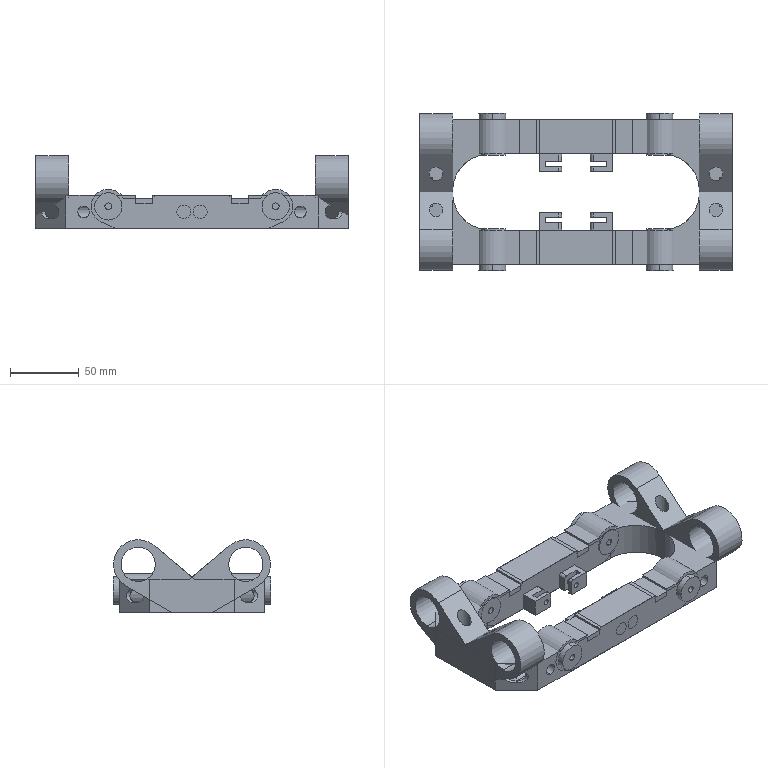NC program | Mastercam | posted with a generic post | part box 228 x 114.503 x 53 mm
Lines 2708 to 3806 of 27132:
(10 FEM |TOOL - 10|DIA. OFF. - 10|LEN. - 10|TOOL DIA. - 10.)
N5468 T10 M6
N5470 G0 G54 G90 X14.273 Y-4.51 C0. B0. S8000 M3
N5472 G43 H10 Z50.
N5474 Z5.
N5476 G1 Z-.5 F600.
N5478 Y-3.51 F4000.
N5480 G3 X13.273 Y-2.51 I-1.
N5482 G1 X3.684
N5484 X-3.024 Y-8.139
N5486 G3 X-3.381 Y-8.905 I.642 J-.766
N5488 X-3.148 Y-9.548 I.999
N5490 G1 X-2.505 Y-10.314
N5492 X14.273 Y-4.51
N5494 Z-1. F600.
N5496 Y-3.51 F4000.
N5498 G3 X13.273 Y-2.51 I-1.
N5500 G1 X3.684
N5502 X-3.024 Y-8.139
N5504 G3 X-3.381 Y-8.905 I.642 J-.766
N5506 X-3.148 Y-9.548 I.999
N5508 G1 X-2.505 Y-10.314
N5510 X14.273 Y-4.51
N5512 Z-1.5 F600.
N5514 Y-3.51 F4000.
N5516 G3 X13.273 Y-2.51 I-1.
N5518 G1 X3.684
N5520 X-3.024 Y-8.139
N5522 G3 X-3.381 Y-8.905 I.642 J-.766
N5524 X-3.148 Y-9.548 I.999
N5526 G1 X-2.505 Y-10.314
N5528 X14.273 Y-4.51
N5530 Z-2. F600.
N5532 Y-3.51 F4000.
N5534 G3 X13.273 Y-2.51 I-1.
N5536 G1 X3.684
N5538 X-3.024 Y-8.139
N5540 G3 X-3.381 Y-8.905 I.642 J-.766
N5542 X-3.148 Y-9.548 I.999
N5544 G1 X-2.505 Y-10.314
N5546 X14.273 Y-4.51
N5548 Z-2.5 F600.
N5550 Y-3.51 F4000.
N5552 G3 X13.273 Y-2.51 I-1.
N5554 G1 X3.684
N5556 X-3.024 Y-8.139
N5558 G3 X-3.381 Y-8.905 I.642 J-.766
N5560 X-3.148 Y-9.548 I.999
N5562 G1 X-2.505 Y-10.314
N5564 X14.273 Y-4.51
N5566 Z-3. F600.
N5568 Y-3.51 F4000.
N5570 G3 X13.273 Y-2.51 I-1.
N5572 G1 X3.684
N5574 X-3.024 Y-8.139
N5576 G3 X-3.381 Y-8.905 I.642 J-.766
N5578 X-3.148 Y-9.548 I.999
N5580 G1 X-2.505 Y-10.314
N5582 X14.273 Y-4.51
N5584 Z-3.5 F600.
N5586 Y-3.51 F4000.
N5588 G3 X13.273 Y-2.51 I-1.
N5590 G1 X3.684
N5592 X-3.024 Y-8.139
N5594 G3 X-3.381 Y-8.905 I.642 J-.766
N5596 X-3.148 Y-9.548 I.999
N5598 G1 X-2.505 Y-10.314
N5600 X14.273 Y-4.51
N5602 Z-4. F600.
N5604 Y-3.51 F4000.
N5606 G3 X13.273 Y-2.51 I-1.
N5608 G1 X3.684
N5610 X-3.024 Y-8.139
N5612 G3 X-3.381 Y-8.905 I.642 J-.766
N5614 X-3.148 Y-9.548 I.999
N5616 G1 X-2.505 Y-10.314
N5618 X14.273 Y-4.51
N5620 Z-4.5 F600.
N5622 Y-3.51 F4000.
N5624 G3 X13.273 Y-2.51 I-1.
N5626 G1 X3.684
N5628 X-3.024 Y-8.139
N5630 G3 X-3.381 Y-8.905 I.642 J-.766
N5632 X-3.148 Y-9.548 I.999
N5634 G1 X-2.505 Y-10.314
N5636 X14.273 Y-4.51
N5638 Z-5. F600.
N5640 Y-3.51 F4000.
N5642 G3 X13.273 Y-2.51 I-1.
N5644 G1 X3.684
N5646 X-3.024 Y-8.139
N5648 G3 X-3.381 Y-8.905 I.642 J-.766
N5650 X-3.148 Y-9.548 I.999
N5652 G1 X-2.505 Y-10.314
N5654 X14.273 Y-4.51
N5656 Z-5.5 F600.
N5658 Y-3.51 F4000.
N5660 G3 X13.273 Y-2.51 I-1.
N5662 G1 X3.684
N5664 X-3.024 Y-8.139
N5666 G3 X-3.381 Y-8.905 I.642 J-.766
N5668 X-3.148 Y-9.548 I.999
N5670 G1 X-2.505 Y-10.314
N5672 X14.273 Y-4.51
N5674 Z-6. F600.
N5676 Y-3.51 F4000.
N5678 G3 X13.273 Y-2.51 I-1.
N5680 G1 X3.684
N5682 X-3.024 Y-8.139
N5684 G3 X-3.381 Y-8.905 I.642 J-.766
N5686 X-3.148 Y-9.548 I.999
N5688 G1 X-2.505 Y-10.314
N5690 X14.273 Y-4.51
N5692 Z-6.5 F600.
N5694 Y-3.51 F4000.
N5696 G3 X13.273 Y-2.51 I-1.
N5698 G1 X3.684
N5700 X-3.024 Y-8.139
N5702 G3 X-3.381 Y-8.905 I.642 J-.766
N5704 X-3.148 Y-9.548 I.999
N5706 G1 X-2.505 Y-10.314
N5708 X14.273 Y-4.51
N5710 Z-7. F600.
N5712 Y-3.51 F4000.
N5714 G3 X13.273 Y-2.51 I-1.
N5716 G1 X3.684
N5718 X-3.024 Y-8.139
N5720 G3 X-3.381 Y-8.905 I.642 J-.766
N5722 X-3.148 Y-9.548 I.999
N5724 G1 X-2.505 Y-10.314
N5726 X14.273 Y-4.51
N5728 Z-7.5 F600.
N5730 Y-3.51 F4000.
N5732 G3 X13.273 Y-2.51 I-1.
N5734 G1 X3.684
N5736 X-3.024 Y-8.139
N5738 G3 X-3.381 Y-8.905 I.642 J-.766
N5740 X-3.148 Y-9.548 I.999
N5742 G1 X-2.505 Y-10.314
N5744 X14.273 Y-4.51
N5746 Z-8. F600.
N5748 Y-3.51 F4000.
N5750 G3 X13.273 Y-2.51 I-1.
N5752 G1 X3.684
N5754 X-3.024 Y-8.139
N5756 G3 X-3.381 Y-8.905 I.642 J-.766
N5758 X-3.148 Y-9.548 I.999
N5760 G1 X-2.505 Y-10.314
N5762 X14.273 Y-4.51
N5764 Z-8.5 F600.
N5766 Y-3.51 F4000.
N5768 G3 X13.273 Y-2.51 I-1.
N5770 G1 X3.684
N5772 X-3.024 Y-8.139
N5774 G3 X-3.381 Y-8.905 I.642 J-.766
N5776 X-3.148 Y-9.548 I.999
N5778 G1 X-2.505 Y-10.314
N5780 X14.273 Y-4.51
N5782 Z-9. F600.
N5784 Y-3.51 F4000.
N5786 G3 X13.273 Y-2.51 I-1.
N5788 G1 X3.684
N5790 X-3.024 Y-8.139
N5792 G3 X-3.381 Y-8.905 I.642 J-.766
N5794 X-3.148 Y-9.548 I.999
N5796 G1 X-2.505 Y-10.314
N5798 X14.273 Y-4.51
N5800 Z-9.5 F600.
N5802 Y-3.51 F4000.
N5804 G3 X13.273 Y-2.51 I-1.
N5806 G1 X3.684
N5808 X-3.024 Y-8.139
N5810 G3 X-3.381 Y-8.905 I.642 J-.766
N5812 X-3.148 Y-9.548 I.999
N5814 G1 X-2.505 Y-10.314
N5816 X14.273 Y-4.51
N5818 Z-10. F600.
N5820 Y-3.51 F4000.
N5822 G3 X13.273 Y-2.51 I-1.
N5824 G1 X3.684
N5826 X-3.024 Y-8.139
N5828 G3 X-3.381 Y-8.905 I.642 J-.766
N5830 X-3.148 Y-9.548 I.999
N5832 G1 X-2.505 Y-10.314
N5834 X14.273 Y-4.51
N5836 Z-10.5 F600.
N5838 Y-3.51 F4000.
N5840 G3 X13.273 Y-2.51 I-1.
N5842 G1 X3.684
N5844 X-3.024 Y-8.139
N5846 G3 X-3.381 Y-8.905 I.642 J-.766
N5848 X-3.148 Y-9.548 I.999
N5850 G1 X-2.505 Y-10.314
N5852 X14.273 Y-4.51
N5854 Z-11. F600.
N5856 Y-3.51 F4000.
N5858 G3 X13.273 Y-2.51 I-1.
N5860 G1 X3.684
N5862 X-3.024 Y-8.139
N5864 G3 X-3.381 Y-8.905 I.642 J-.766
N5866 X-3.148 Y-9.548 I.999
N5868 G1 X-2.505 Y-10.314
N5870 X14.273 Y-4.51
N5872 Z-11.5 F600.
N5874 Y-3.51 F4000.
N5876 G3 X13.273 Y-2.51 I-1.
N5878 G1 X3.684
N5880 X-3.024 Y-8.139
N5882 G3 X-3.381 Y-8.905 I.642 J-.766
N5884 X-3.148 Y-9.548 I.999
N5886 G1 X-2.505 Y-10.314
N5888 X14.273 Y-4.51
N5890 Z-12. F600.
N5892 Y-3.51 F4000.
N5894 G3 X13.273 Y-2.51 I-1.
N5896 G1 X3.684
N5898 X-3.024 Y-8.139
N5900 G3 X-3.381 Y-8.905 I.642 J-.766
N5902 X-3.148 Y-9.548 I.999
N5904 G1 X-2.505 Y-10.314
N5906 X14.273 Y-4.51
N5908 Z-12.5 F600.
N5910 Y-3.51 F4000.
N5912 G3 X13.273 Y-2.51 I-1.
N5914 G1 X3.684
N5916 X-3.024 Y-8.139
N5918 G3 X-3.381 Y-8.905 I.642 J-.766
N5920 X-3.148 Y-9.548 I.999
N5922 G1 X-2.505 Y-10.314
N5924 X14.273 Y-4.51
N5926 Z-13. F600.
N5928 Y-3.51 F4000.
N5930 G3 X13.273 Y-2.51 I-1.
N5932 G1 X3.684
N5934 X-3.024 Y-8.139
N5936 G3 X-3.381 Y-8.905 I.642 J-.766
N5938 X-3.148 Y-9.548 I.999
N5940 G1 X-2.505 Y-10.314
N5942 X14.273 Y-4.51
N5944 Z-13.5 F600.
N5946 Y-3.51 F4000.
N5948 G3 X13.273 Y-2.51 I-1.
N5950 G1 X3.684
N5952 X-3.024 Y-8.139
N5954 G3 X-3.381 Y-8.905 I.642 J-.766
N5956 X-3.148 Y-9.548 I.999
N5958 G1 X-2.505 Y-10.314
N5960 X14.273 Y-4.51
N5962 Z-14. F600.
N5964 Y-3.51 F4000.
N5966 G3 X13.273 Y-2.51 I-1.
N5968 G1 X3.684
N5970 X-3.024 Y-8.139
N5972 G3 X-3.381 Y-8.905 I.642 J-.766
N5974 X-3.148 Y-9.548 I.999
N5976 G1 X-2.505 Y-10.314
N5978 X14.273 Y-4.51
N5980 Z-14.5 F600.
N5982 Y-3.51 F4000.
N5984 G3 X13.273 Y-2.51 I-1.
N5986 G1 X3.684
N5988 X-3.024 Y-8.139
N5990 G3 X-3.381 Y-8.905 I.642 J-.766
N5992 X-3.148 Y-9.548 I.999
N5994 G1 X-2.505 Y-10.314
N5996 X14.273 Y-4.51
N5998 Z-15. F600.
N6000 Y-3.51 F4000.
N6002 G3 X13.273 Y-2.51 I-1.
N6004 G1 X3.684
N6006 X-3.024 Y-8.139
N6008 G3 X-3.381 Y-8.905 I.642 J-.766
N6010 X-3.148 Y-9.548 I.999
N6012 G1 X-2.505 Y-10.314
N6014 X14.273 Y-4.51
N6016 Z-15.5 F600.
N6018 Y-3.51 F4000.
N6020 G3 X13.273 Y-2.51 I-1.
N6022 G1 X3.684
N6024 X-3.024 Y-8.139
N6026 G3 X-3.381 Y-8.905 I.642 J-.766
N6028 X-3.148 Y-9.548 I.999
N6030 G1 X-2.505 Y-10.314
N6032 X14.273 Y-4.51
N6034 Z-16. F600.
N6036 Y-3.51 F4000.
N6038 G3 X13.273 Y-2.51 I-1.
N6040 G1 X3.684
N6042 X-3.024 Y-8.139
N6044 G3 X-3.381 Y-8.905 I.642 J-.766
N6046 X-3.148 Y-9.548 I.999
N6048 G1 X-2.505 Y-10.314
N6050 X14.273 Y-4.51
N6052 Z-16.5 F600.
N6054 Y-3.51 F4000.
N6056 G3 X13.273 Y-2.51 I-1.
N6058 G1 X3.684
N6060 X-3.024 Y-8.139
N6062 G3 X-3.381 Y-8.905 I.642 J-.766
N6064 X-3.148 Y-9.548 I.999
N6066 G1 X-2.505 Y-10.314
N6068 X14.273 Y-4.51
N6070 Z-17. F600.
N6072 Y-3.51 F4000.
N6074 G3 X13.273 Y-2.51 I-1.
N6076 G1 X3.684
N6078 X-3.024 Y-8.139
N6080 G3 X-3.381 Y-8.905 I.642 J-.766
N6082 X-3.148 Y-9.548 I.999
N6084 G1 X-2.505 Y-10.314
N6086 X14.273 Y-4.51
N6088 Z-17.5 F600.
N6090 Y-3.51 F4000.
N6092 G3 X13.273 Y-2.51 I-1.
N6094 G1 X3.684
N6096 X-3.024 Y-8.139
N6098 G3 X-3.381 Y-8.905 I.642 J-.766
N6100 X-3.148 Y-9.548 I.999
N6102 G1 X-2.505 Y-10.314
N6104 X14.273 Y-4.51
N6106 Z-18. F600.
N6108 Y-3.51 F4000.
N6110 G3 X13.273 Y-2.51 I-1.
N6112 G1 X3.684
N6114 X-3.024 Y-8.139
N6116 G3 X-3.381 Y-8.905 I.642 J-.766
N6118 X-3.148 Y-9.548 I.999
N6120 G1 X-2.505 Y-10.314
N6122 X14.273 Y-4.51
N6124 Z-18.5 F600.
N6126 Y-3.51 F4000.
N6128 G3 X13.273 Y-2.51 I-1.
N6130 G1 X3.684
N6132 X-3.024 Y-8.139
N6134 G3 X-3.381 Y-8.905 I.642 J-.766
N6136 X-3.148 Y-9.548 I.999
N6138 G1 X-2.505 Y-10.314
N6140 X14.273 Y-4.51
N6142 Z-19. F600.
N6144 Y-3.51 F4000.
N6146 G3 X13.273 Y-2.51 I-1.
N6148 G1 X3.684
N6150 X-3.024 Y-8.139
N6152 G3 X-3.381 Y-8.905 I.642 J-.766
N6154 X-3.148 Y-9.548 I.999
N6156 G1 X-2.505 Y-10.314
N6158 X14.273 Y-4.51
N6160 Z-19.5 F600.
N6162 Y-3.51 F4000.
N6164 G3 X13.273 Y-2.51 I-1.
N6166 G1 X3.684
N6168 X-3.024 Y-8.139
N6170 G3 X-3.381 Y-8.905 I.642 J-.766
N6172 X-3.148 Y-9.548 I.999
N6174 G1 X-2.505 Y-10.314
N6176 X14.273 Y-4.51
N6178 Z-20. F600.
N6180 Y-3.51 F4000.
N6182 G3 X13.273 Y-2.51 I-1.
N6184 G1 X3.684
N6186 X-3.024 Y-8.139
N6188 G3 X-3.381 Y-8.905 I.642 J-.766
N6190 X-3.148 Y-9.548 I.999
N6192 G1 X-2.505 Y-10.314
N6194 X14.273 Y-4.51
N6196 Z-20.5 F600.
N6198 Y-3.51 F4000.
N6200 G3 X13.273 Y-2.51 I-1.
N6202 G1 X3.684
N6204 X-3.024 Y-8.139
N6206 G3 X-3.381 Y-8.905 I.642 J-.766
N6208 X-3.148 Y-9.548 I.999
N6210 G1 X-2.505 Y-10.314
N6212 X14.273 Y-4.51
N6214 Z-21. F600.
N6216 Y-3.51 F4000.
N6218 G3 X13.273 Y-2.51 I-1.
N6220 G1 X3.684
N6222 X-3.024 Y-8.139
N6224 G3 X-3.381 Y-8.905 I.642 J-.766
N6226 X-3.148 Y-9.548 I.999
N6228 G1 X-2.505 Y-10.314
N6230 X14.273 Y-4.51
N6232 Z-21.5 F600.
N6234 Y-3.51 F4000.
N6236 G3 X13.273 Y-2.51 I-1.
N6238 G1 X3.684
N6240 X-3.024 Y-8.139
N6242 G3 X-3.381 Y-8.905 I.642 J-.766
N6244 X-3.148 Y-9.548 I.999
N6246 G1 X-2.505 Y-10.314
N6248 X14.273 Y-4.51
N6250 Z-22. F600.
N6252 Y-3.51 F4000.
N6254 G3 X13.273 Y-2.51 I-1.
N6256 G1 X3.684
N6258 X-3.024 Y-8.139
N6260 G3 X-3.381 Y-8.905 I.642 J-.766
N6262 X-3.148 Y-9.548 I.999
N6264 G1 X-2.505 Y-10.314
N6266 X14.273 Y-4.51
N6268 Z-22.5 F600.
N6270 Y-3.51 F4000.
N6272 G3 X13.273 Y-2.51 I-1.
N6274 G1 X3.684
N6276 X-3.024 Y-8.139
N6278 G3 X-3.381 Y-8.905 I.642 J-.766
N6280 X-3.148 Y-9.548 I.999
N6282 G1 X-2.505 Y-10.314
N6284 X14.273 Y-4.51
N6286 Z-23. F600.
N6288 Y-3.51 F4000.
N6290 G3 X13.273 Y-2.51 I-1.
N6292 G1 X3.684
N6294 X-3.024 Y-8.139
N6296 G3 X-3.381 Y-8.905 I.642 J-.766
N6298 X-3.148 Y-9.548 I.999
N6300 G1 X-2.505 Y-10.314
N6302 X14.273 Y-4.51
N6304 Z-23.5 F600.
N6306 Y-3.51 F4000.
N6308 G3 X13.273 Y-2.51 I-1.
N6310 G1 X3.684
N6312 X-3.024 Y-8.139
N6314 G3 X-3.381 Y-8.905 I.642 J-.766
N6316 X-3.148 Y-9.548 I.999
N6318 G1 X-2.505 Y-10.314
N6320 X14.273 Y-4.51
N6322 Z-24. F600.
N6324 Y-3.51 F4000.
N6326 G3 X13.273 Y-2.51 I-1.
N6328 G1 X3.684
N6330 X-3.024 Y-8.139
N6332 G3 X-3.381 Y-8.905 I.642 J-.766
N6334 X-3.148 Y-9.548 I.999
N6336 G1 X-2.505 Y-10.314
N6338 X14.273 Y-4.51
N6340 Z-24.5 F600.
N6342 Y-3.51 F4000.
N6344 G3 X13.273 Y-2.51 I-1.
N6346 G1 X3.684
N6348 X-3.024 Y-8.139
N6350 G3 X-3.381 Y-8.905 I.642 J-.766
N6352 X-3.148 Y-9.548 I.999
N6354 G1 X-2.505 Y-10.314
N6356 X14.273 Y-4.51
N6358 Z-25. F600.
N6360 Y-3.51 F4000.
N6362 G3 X13.273 Y-2.51 I-1.
N6364 G1 X3.684
N6366 X-3.024 Y-8.139
N6368 G3 X-3.381 Y-8.905 I.642 J-.766
N6370 X-3.148 Y-9.548 I.999
N6372 G1 X-2.505 Y-10.314
N6374 X14.273 Y-4.51
N6376 Z-25.5 F600.
N6378 Y-3.51 F4000.
N6380 G3 X13.273 Y-2.51 I-1.
N6382 G1 X3.684
N6384 X-3.024 Y-8.139
N6386 G3 X-3.381 Y-8.905 I.642 J-.766
N6388 X-3.148 Y-9.548 I.999
N6390 G1 X-2.505 Y-10.314
N6392 X14.273 Y-4.51
N6394 Z-26. F600.
N6396 Y-3.51 F4000.
N6398 G3 X13.273 Y-2.51 I-1.
N6400 G1 X3.684
N6402 X-3.024 Y-8.139
N6404 G3 X-3.381 Y-8.905 I.642 J-.766
N6406 X-3.148 Y-9.548 I.999
N6408 G1 X-2.505 Y-10.314
N6410 G0 Z50.
N6412 S6000 M3
N6414 X64.338 Y27.5
N6416 Z5.
N6418 G1 Z-26. F600.
N6420 X63.338 F1000.
N6422 G3 X62.338 Y26.5 J-1.
N6424 G1 Y2.5
N6426 G2 X57.248 Y-2.59 I-5.09
N6428 G1 X3.713
N6430 X-24.41 Y-26.188
N6432 G2 X-39.252 Y-31.59 I-14.842 J17.688
N6434 X-62.342 Y-8.5 J23.09
N6436 X-50.797 Y11.497 I23.09
N6438 G1 X-15.994 Y31.59
N6440 X57.248
N6442 G2 X62.338 Y26.5 J-5.09
N6444 G1 Y21.5
N6446 G3 X63.338 Y20.5 I1.
N6448 G1 X64.338
N6450 G0 Z24.
N6452 X64.238 Y27.5
N6454 Z5.
N6456 G1 Z-26. F600.
N6458 X63.238 F1000.
N6460 G3 X62.238 Y26.5 J-1.
N6462 G1 Y2.5
N6464 G2 X57.248 Y-2.49 I-4.99
N6466 G1 X3.68
N6468 X3.674 Y-2.492
N6470 X-24.474 Y-26.111
N6472 G2 X-39.252 Y-31.49 I-14.778 J17.611
N6474 X-62.242 Y-8.5 J22.99
N6476 X-50.747 Y11.41 I22.99
N6478 G1 X-15.967 Y31.49
N6480 X57.248
N6482 G2 X62.238 Y26.5 J-4.99
N6484 G1 Y21.5
N6486 G3 X63.238 Y20.5 I1.
N6488 G1 X64.238
N6490 G0 Z50.
N6492 S8000 M3
N6494 X-38.252 Y-7.1
N6496 Z5.
N6498 G1 Z0. F600.
N6500 Y-6.1 F4000.
N6502 G3 X-39.252 Y-5.1 I-1.
N6504 X-42.652 Y-8.5 Z-.125 J-3.4
N6506 X-39.252 Y-11.9 Z-.25 I3.4
N6508 X-35.852 Y-8.5 Z-.375 J3.4
N6510 X-39.252 Y-5.1 Z-.5 I-3.4
N6512 X-42.652 Y-8.5 Z-.625 J-3.4
N6514 X-39.252 Y-11.9 Z-.75 I3.4
N6516 X-35.852 Y-8.5 Z-.875 J3.4
N6518 X-39.252 Y-5.1 Z-1. I-3.4
N6520 X-42.652 Y-8.5 Z-1.125 J-3.4
N6522 X-39.252 Y-11.9 Z-1.25 I3.4
N6524 X-35.852 Y-8.5 Z-1.375 J3.4
N6526 X-39.252 Y-5.1 Z-1.5 I-3.4
N6528 X-42.652 Y-8.5 Z-1.625 J-3.4
N6530 X-39.252 Y-11.9 Z-1.75 I3.4
N6532 X-35.852 Y-8.5 Z-1.875 J3.4
N6534 X-39.252 Y-5.1 Z-2. I-3.4
N6536 X-42.652 Y-8.5 Z-2.125 J-3.4
N6538 X-39.252 Y-11.9 Z-2.25 I3.4
N6540 X-35.852 Y-8.5 Z-2.375 J3.4
N6542 X-39.252 Y-5.1 Z-2.5 I-3.4
N6544 X-42.652 Y-8.5 Z-2.625 J-3.4
N6546 X-39.252 Y-11.9 Z-2.75 I3.4
N6548 X-35.852 Y-8.5 Z-2.875 J3.4
N6550 X-39.252 Y-5.1 Z-3. I-3.4
N6552 X-42.652 Y-8.5 Z-3.125 J-3.4
N6554 X-39.252 Y-11.9 Z-3.25 I3.4
N6556 X-35.852 Y-8.5 Z-3.375 J3.4
N6558 X-39.252 Y-5.1 Z-3.5 I-3.4
N6560 X-42.652 Y-8.5 Z-3.625 J-3.4
N6562 X-39.252 Y-11.9 Z-3.75 I3.4
N6564 X-35.852 Y-8.5 Z-3.875 J3.4
N6566 X-39.252 Y-5.1 Z-4. I-3.4
N6568 X-42.652 Y-8.5 Z-4.125 J-3.4
N6570 X-39.252 Y-11.9 Z-4.25 I3.4
N6572 X-35.852 Y-8.5 Z-4.375 J3.4
N6574 X-39.252 Y-5.1 Z-4.5 I-3.4
N6576 X-42.652 Y-8.5 Z-4.625 J-3.4
N6578 X-39.252 Y-11.9 Z-4.75 I3.4
N6580 X-35.852 Y-8.5 Z-4.875 J3.4
N6582 X-39.252 Y-5.1 Z-5. I-3.4
N6584 X-42.652 Y-8.5 Z-5.125 J-3.4
N6586 X-39.252 Y-11.9 Z-5.25 I3.4
N6588 X-35.852 Y-8.5 Z-5.375 J3.4
N6590 X-39.252 Y-5.1 Z-5.5 I-3.4
N6592 X-42.652 Y-8.5 Z-5.625 J-3.4
N6594 X-39.252 Y-11.9 Z-5.75 I3.4
N6596 X-35.852 Y-8.5 Z-5.875 J3.4
N6598 X-39.252 Y-5.1 Z-6. I-3.4
N6600 X-42.652 Y-8.5 Z-6.125 J-3.4
N6602 X-39.252 Y-11.9 Z-6.25 I3.4
N6604 X-35.852 Y-8.5 Z-6.375 J3.4
N6606 X-39.252 Y-5.1 Z-6.5 I-3.4
N6608 X-42.652 Y-8.5 Z-6.625 J-3.4
N6610 X-39.252 Y-11.9 Z-6.75 I3.4
N6612 X-35.852 Y-8.5 Z-6.875 J3.4
N6614 X-39.252 Y-5.1 Z-7. I-3.4
N6616 X-42.652 Y-8.5 Z-7.125 J-3.4
N6618 X-39.252 Y-11.9 Z-7.25 I3.4
N6620 X-35.852 Y-8.5 Z-7.375 J3.4
N6622 X-39.252 Y-5.1 Z-7.5 I-3.4
N6624 X-42.652 Y-8.5 Z-7.625 J-3.4
N6626 X-39.252 Y-11.9 Z-7.75 I3.4
N6628 X-35.852 Y-8.5 Z-7.875 J3.4
N6630 X-39.252 Y-5.1 Z-8. I-3.4
N6632 X-42.652 Y-8.5 Z-8.125 J-3.4
N6634 X-39.252 Y-11.9 Z-8.25 I3.4
N6636 X-35.852 Y-8.5 Z-8.375 J3.4
N6638 X-39.252 Y-5.1 Z-8.5 I-3.4
N6640 X-42.652 Y-8.5 Z-8.625 J-3.4
N6642 X-39.252 Y-11.9 Z-8.75 I3.4
N6644 X-35.852 Y-8.5 Z-8.875 J3.4
N6646 X-39.252 Y-5.1 Z-9. I-3.4
N6648 X-42.652 Y-8.5 Z-9.125 J-3.4
N6650 X-39.252 Y-11.9 Z-9.25 I3.4
N6652 X-35.852 Y-8.5 Z-9.375 J3.4
N6654 X-39.252 Y-5.1 Z-9.5 I-3.4
N6656 X-42.652 Y-8.5 Z-9.625 J-3.4
N6658 X-39.252 Y-11.9 Z-9.75 I3.4
N6660 X-35.852 Y-8.5 Z-9.875 J3.4
N6662 X-39.252 Y-5.1 Z-10. I-3.4
N6664 X-42.652 Y-8.5 Z-10.125 J-3.4
N6666 X-39.252 Y-11.9 Z-10.25 I3.4
N6668 X-35.852 Y-8.5 Z-10.375 J3.4
N6670 X-39.252 Y-5.1 Z-10.5 I-3.4
N6672 X-42.652 Y-8.5 Z-10.625 J-3.4
N6674 X-39.252 Y-11.9 Z-10.75 I3.4
N6676 X-35.852 Y-8.5 Z-10.875 J3.4
N6678 X-39.252 Y-5.1 Z-11. I-3.4
N6680 X-42.652 Y-8.5 Z-11.125 J-3.4
N6682 X-39.252 Y-11.9 Z-11.25 I3.4
N6684 X-35.852 Y-8.5 Z-11.375 J3.4
N6686 X-39.252 Y-5.1 Z-11.5 I-3.4
N6688 X-42.652 Y-8.5 Z-11.625 J-3.4
N6690 X-39.252 Y-11.9 Z-11.75 I3.4
N6692 X-35.852 Y-8.5 Z-11.875 J3.4
N6694 X-39.252 Y-5.1 Z-12. I-3.4
N6696 X-42.652 Y-8.5 Z-12.125 J-3.4
N6698 X-39.252 Y-11.9 Z-12.25 I3.4
N6700 X-35.852 Y-8.5 Z-12.375 J3.4
N6702 X-39.252 Y-5.1 Z-12.5 I-3.4
N6704 X-42.652 Y-8.5 Z-12.625 J-3.4
N6706 X-39.252 Y-11.9 Z-12.75 I3.4
N6708 X-35.852 Y-8.5 Z-12.875 J3.4
N6710 X-39.252 Y-5.1 Z-13. I-3.4
N6712 X-42.652 Y-8.5 Z-13.125 J-3.4
N6714 X-39.252 Y-11.9 Z-13.25 I3.4
N6716 X-35.852 Y-8.5 Z-13.375 J3.4
N6718 X-39.252 Y-5.1 Z-13.5 I-3.4
N6720 X-42.652 Y-8.5 Z-13.625 J-3.4
N6722 X-39.252 Y-11.9 Z-13.75 I3.4
N6724 X-35.852 Y-8.5 Z-13.875 J3.4
N6726 X-39.252 Y-5.1 Z-14. I-3.4
N6728 X-42.652 Y-8.5 Z-14.125 J-3.4
N6730 X-39.252 Y-11.9 Z-14.25 I3.4
N6732 X-35.852 Y-8.5 Z-14.375 J3.4
N6734 X-39.252 Y-5.1 Z-14.5 I-3.4
N6736 X-42.652 Y-8.5 Z-14.625 J-3.4
N6738 X-39.252 Y-11.9 Z-14.75 I3.4
N6740 X-35.852 Y-8.5 Z-14.875 J3.4
N6742 X-39.252 Y-5.1 Z-15. I-3.4
N6744 X-42.652 Y-8.5 Z-15.125 J-3.4
N6746 X-39.252 Y-11.9 Z-15.25 I3.4
N6748 X-35.852 Y-8.5 Z-15.375 J3.4
N6750 X-39.252 Y-5.1 Z-15.5 I-3.4
N6752 X-42.652 Y-8.5 Z-15.625 J-3.4
N6754 X-39.252 Y-11.9 Z-15.75 I3.4
N6756 X-35.852 Y-8.5 Z-15.875 J3.4
N6758 X-39.252 Y-5.1 Z-16. I-3.4
N6760 X-42.652 Y-8.5 Z-16.125 J-3.4
N6762 X-39.252 Y-11.9 Z-16.25 I3.4
N6764 X-35.852 Y-8.5 Z-16.375 J3.4
N6766 X-39.252 Y-5.1 Z-16.5 I-3.4
N6768 X-42.652 Y-8.5 Z-16.625 J-3.4
N6770 X-39.252 Y-11.9 Z-16.75 I3.4
N6772 X-35.852 Y-8.5 Z-16.875 J3.4
N6774 X-39.252 Y-5.1 Z-17. I-3.4
N6776 X-42.652 Y-8.5 Z-17.125 J-3.4
N6778 X-39.252 Y-11.9 Z-17.25 I3.4
N6780 X-35.852 Y-8.5 Z-17.375 J3.4
N6782 X-39.252 Y-5.1 Z-17.5 I-3.4
N6784 X-42.652 Y-8.5 Z-17.625 J-3.4
N6786 X-39.252 Y-11.9 Z-17.75 I3.4
N6788 X-35.852 Y-8.5 Z-17.875 J3.4
N6790 X-39.252 Y-5.1 Z-18. I-3.4
N6792 X-42.652 Y-8.5 Z-18.125 J-3.4
N6794 X-39.252 Y-11.9 Z-18.25 I3.4
N6796 X-35.852 Y-8.5 Z-18.375 J3.4
N6798 X-39.252 Y-5.1 Z-18.5 I-3.4
N6800 X-42.652 Y-8.5 Z-18.625 J-3.4
N6802 X-39.252 Y-11.9 Z-18.75 I3.4
N6804 X-35.852 Y-8.5 Z-18.875 J3.4
N6806 X-39.252 Y-5.1 Z-19. I-3.4
N6808 X-42.652 Y-8.5 Z-19.125 J-3.4
N6810 X-39.252 Y-11.9 Z-19.25 I3.4
N6812 X-35.852 Y-8.5 Z-19.375 J3.4
N6814 X-39.252 Y-5.1 Z-19.5 I-3.4
N6816 X-42.652 Y-8.5 Z-19.625 J-3.4
N6818 X-39.252 Y-11.9 Z-19.75 I3.4
N6820 X-35.852 Y-8.5 Z-19.875 J3.4
N6822 X-39.252 Y-5.1 Z-20. I-3.4
N6824 X-42.652 Y-8.5 Z-20.125 J-3.4
N6826 X-39.252 Y-11.9 Z-20.25 I3.4
N6828 X-35.852 Y-8.5 Z-20.375 J3.4
N6830 X-39.252 Y-5.1 Z-20.5 I-3.4
N6832 X-42.652 Y-8.5 Z-20.625 J-3.4
N6834 X-39.252 Y-11.9 Z-20.75 I3.4
N6836 X-35.852 Y-8.5 Z-20.875 J3.4
N6838 X-39.252 Y-5.1 Z-21. I-3.4
N6840 X-42.652 Y-8.5 Z-21.125 J-3.4
N6842 X-39.252 Y-11.9 Z-21.25 I3.4
N6844 X-35.852 Y-8.5 Z-21.375 J3.4
N6846 X-39.252 Y-5.1 Z-21.5 I-3.4
N6848 X-42.652 Y-8.5 Z-21.625 J-3.4
N6850 X-39.252 Y-11.9 Z-21.75 I3.4
N6852 X-35.852 Y-8.5 Z-21.875 J3.4
N6854 X-39.252 Y-5.1 Z-22. I-3.4
N6856 X-42.652 Y-8.5 Z-22.125 J-3.4
N6858 X-39.252 Y-11.9 Z-22.25 I3.4
N6860 X-35.852 Y-8.5 Z-22.375 J3.4
N6862 X-39.252 Y-5.1 Z-22.5 I-3.4
N6864 X-42.652 Y-8.5 Z-22.625 J-3.4
N6866 X-39.252 Y-11.9 Z-22.75 I3.4
N6868 X-35.852 Y-8.5 Z-22.875 J3.4
N6870 X-39.252 Y-5.1 Z-23. I-3.4
N6872 X-42.652 Y-8.5 Z-23.125 J-3.4
N6874 X-39.252 Y-11.9 Z-23.25 I3.4
N6876 X-35.852 Y-8.5 Z-23.375 J3.4
N6878 X-39.252 Y-5.1 Z-23.5 I-3.4
N6880 X-42.652 Y-8.5 Z-23.625 J-3.4
N6882 X-39.252 Y-11.9 Z-23.75 I3.4
N6884 X-35.852 Y-8.5 Z-23.875 J3.4
N6886 X-39.252 Y-5.1 Z-24. I-3.4
N6888 X-42.652 Y-8.5 Z-24.125 J-3.4
N6890 X-39.252 Y-11.9 Z-24.25 I3.4
N6892 X-35.852 Y-8.5 Z-24.375 J3.4
N6894 X-39.252 Y-5.1 Z-24.5 I-3.4
N6896 X-42.652 Y-8.5 Z-24.625 J-3.4
N6898 X-39.252 Y-11.9 Z-24.75 I3.4
N6900 X-35.852 Y-8.5 Z-24.875 J3.4
N6902 X-39.252 Y-5.1 Z-25. I-3.4
N6904 X-42.652 Y-8.5 Z-25.125 J-3.4
N6906 X-39.252 Y-11.9 Z-25.25 I3.4
N6908 X-35.852 Y-8.5 Z-25.375 J3.4
N6910 X-39.252 Y-5.1 Z-25.5 I-3.4
N6912 X-42.652 Y-8.5 Z-25.625 J-3.4
N6914 X-39.252 Y-11.9 Z-25.75 I3.4
N6916 X-35.852 Y-8.5 Z-25.875 J3.4
N6918 X-39.252 Y-5.1 Z-26. I-3.4
N6920 X-42.652 Y-8.5 J-3.4
N6922 X-39.252 Y-11.9 I3.4
N6924 X-35.852 Y-8.5 J3.4
N6926 X-39.252 Y-5.1 I-3.4
N6928 X-42.635 Y-8.16 J-3.4
N6930 X-42.64 Y-8.26 I.995 J-.1
N6932 X-41.74 Y-9.255 I1.
N6934 G1 X-40.745 Y-9.355
N6936 G0 Z24.
N6938 X-38.252 Y-3.1
N6940 Z5.
N6942 G1 Z0. F600.
N6944 Y-2.1 F4000.
N6946 G3 X-39.252 Y-1.1 I-1.
N6948 X-46.652 Y-8.5 Z-.125 J-7.4
N6950 X-39.252 Y-15.9 Z-.25 I7.4
N6952 X-31.852 Y-8.5 Z-.375 J7.4
N6954 X-39.252 Y-1.1 Z-.5 I-7.4
N6956 X-46.652 Y-8.5 Z-.625 J-7.4
N6958 X-39.252 Y-15.9 Z-.75 I7.4
N6960 X-31.852 Y-8.5 Z-.875 J7.4
N6962 X-39.252 Y-1.1 Z-1. I-7.4
N6964 X-46.652 Y-8.5 Z-1.125 J-7.4
N6966 X-39.252 Y-15.9 Z-1.25 I7.4
N6968 X-31.852 Y-8.5 Z-1.375 J7.4
N6970 X-39.252 Y-1.1 Z-1.5 I-7.4
N6972 X-46.652 Y-8.5 Z-1.625 J-7.4
N6974 X-39.252 Y-15.9 Z-1.75 I7.4
N6976 X-31.852 Y-8.5 Z-1.875 J7.4
N6978 X-39.252 Y-1.1 Z-2. I-7.4
N6980 X-46.652 Y-8.5 Z-2.125 J-7.4
N6982 X-39.252 Y-15.9 Z-2.25 I7.4
N6984 X-31.852 Y-8.5 Z-2.375 J7.4
N6986 X-39.252 Y-1.1 Z-2.5 I-7.4
N6988 X-46.652 Y-8.5 Z-2.625 J-7.4
N6990 X-39.252 Y-15.9 Z-2.75 I7.4
N6992 X-31.852 Y-8.5 Z-2.875 J7.4
N6994 X-39.252 Y-1.1 Z-3. I-7.4
N6996 X-46.652 Y-8.5 Z-3.125 J-7.4
N6998 X-39.252 Y-15.9 Z-3.25 I7.4
N7000 X-31.852 Y-8.5 Z-3.375 J7.4
N7002 X-39.252 Y-1.1 Z-3.5 I-7.4
N7004 X-46.652 Y-8.5 Z-3.625 J-7.4
N7006 X-39.252 Y-15.9 Z-3.75 I7.4
N7008 X-31.852 Y-8.5 Z-3.875 J7.4
N7010 X-39.252 Y-1.1 Z-4. I-7.4
N7012 X-46.652 Y-8.5 Z-4.125 J-7.4
N7014 X-39.252 Y-15.9 Z-4.25 I7.4
N7016 X-31.852 Y-8.5 Z-4.375 J7.4
N7018 X-39.252 Y-1.1 Z-4.5 I-7.4
N7020 X-46.652 Y-8.5 Z-4.625 J-7.4
N7022 X-39.252 Y-15.9 Z-4.75 I7.4
N7024 X-31.852 Y-8.5 Z-4.875 J7.4
N7026 X-39.252 Y-1.1 Z-5. I-7.4
N7028 X-46.652 Y-8.5 Z-5.125 J-7.4
N7030 X-39.252 Y-15.9 Z-5.25 I7.4
N7032 X-31.852 Y-8.5 Z-5.375 J7.4
N7034 X-39.252 Y-1.1 Z-5.5 I-7.4
N7036 X-46.652 Y-8.5 Z-5.625 J-7.4
N7038 X-39.252 Y-15.9 Z-5.75 I7.4
N7040 X-31.852 Y-8.5 Z-5.875 J7.4
N7042 X-39.252 Y-1.1 Z-6. I-7.4
N7044 X-46.652 Y-8.5 Z-6.125 J-7.4
N7046 X-39.252 Y-15.9 Z-6.25 I7.4
N7048 X-31.852 Y-8.5 Z-6.375 J7.4
N7050 X-39.252 Y-1.1 Z-6.5 I-7.4
N7052 X-46.652 Y-8.5 Z-6.625 J-7.4
N7054 X-39.252 Y-15.9 Z-6.75 I7.4
N7056 X-31.852 Y-8.5 Z-6.875 J7.4
N7058 X-39.252 Y-1.1 Z-7. I-7.4
N7060 X-46.652 Y-8.5 Z-7.125 J-7.4
N7062 X-39.252 Y-15.9 Z-7.25 I7.4
N7064 X-31.852 Y-8.5 Z-7.375 J7.4
N7066 X-39.252 Y-1.1 Z-7.5 I-7.4
N7068 X-46.652 Y-8.5 Z-7.625 J-7.4
N7070 X-39.252 Y-15.9 Z-7.75 I7.4
N7072 X-31.852 Y-8.5 Z-7.875 J7.4
N7074 X-39.252 Y-1.1 Z-8. I-7.4
N7076 X-46.652 Y-8.5 Z-8.125 J-7.4
N7078 X-39.252 Y-15.9 Z-8.25 I7.4
N7080 X-31.852 Y-8.5 Z-8.375 J7.4
N7082 X-39.252 Y-1.1 Z-8.5 I-7.4
N7084 X-46.652 Y-8.5 Z-8.625 J-7.4
N7086 X-39.252 Y-15.9 Z-8.75 I7.4
N7088 X-31.852 Y-8.5 Z-8.875 J7.4
N7090 X-39.252 Y-1.1 Z-9. I-7.4
N7092 X-46.652 Y-8.5 Z-9.125 J-7.4
N7094 X-39.252 Y-15.9 Z-9.25 I7.4
N7096 X-31.852 Y-8.5 Z-9.375 J7.4
N7098 X-39.252 Y-1.1 Z-9.5 I-7.4
N7100 X-46.652 Y-8.5 Z-9.625 J-7.4
N7102 X-39.252 Y-15.9 Z-9.75 I7.4
N7104 X-31.852 Y-8.5 Z-9.875 J7.4
N7106 X-39.252 Y-1.1 Z-10. I-7.4
N7108 X-46.652 Y-8.5 Z-10.125 J-7.4
N7110 X-39.252 Y-15.9 Z-10.25 I7.4
N7112 X-31.852 Y-8.5 Z-10.375 J7.4
N7114 X-39.252 Y-1.1 Z-10.5 I-7.4
N7116 X-46.652 Y-8.5 Z-10.625 J-7.4
N7118 X-39.252 Y-15.9 Z-10.75 I7.4
N7120 X-31.852 Y-8.5 Z-10.875 J7.4
N7122 X-39.252 Y-1.1 Z-11. I-7.4
N7124 X-46.652 Y-8.5 Z-11.125 J-7.4
N7126 X-39.252 Y-15.9 Z-11.25 I7.4
N7128 X-31.852 Y-8.5 Z-11.375 J7.4
N7130 X-39.252 Y-1.1 Z-11.5 I-7.4
N7132 X-46.652 Y-8.5 Z-11.625 J-7.4
N7134 X-39.252 Y-15.9 Z-11.75 I7.4
N7136 X-31.852 Y-8.5 Z-11.875 J7.4
N7138 X-39.252 Y-1.1 Z-12. I-7.4
N7140 X-46.652 Y-8.5 Z-12.125 J-7.4
N7142 X-39.252 Y-15.9 Z-12.25 I7.4
N7144 X-31.852 Y-8.5 Z-12.375 J7.4
N7146 X-39.252 Y-1.1 Z-12.5 I-7.4
N7148 X-46.652 Y-8.5 Z-12.625 J-7.4
N7150 X-39.252 Y-15.9 Z-12.75 I7.4
N7152 X-31.852 Y-8.5 Z-12.875 J7.4
N7154 X-39.252 Y-1.1 Z-13. I-7.4
N7156 X-46.652 Y-8.5 Z-13.125 J-7.4
N7158 X-39.252 Y-15.9 Z-13.25 I7.4
N7160 X-31.852 Y-8.5 Z-13.375 J7.4
N7162 X-39.252 Y-1.1 Z-13.5 I-7.4
N7164 X-46.652 Y-8.5 Z-13.625 J-7.4
N7166 X-39.252 Y-15.9 Z-13.75 I7.4
N7168 X-31.852 Y-8.5 Z-13.875 J7.4
N7170 X-39.252 Y-1.1 Z-14. I-7.4
N7172 X-46.652 Y-8.5 Z-14.125 J-7.4
N7174 X-39.252 Y-15.9 Z-14.25 I7.4
N7176 X-31.852 Y-8.5 Z-14.375 J7.4
N7178 X-39.252 Y-1.1 Z-14.5 I-7.4
N7180 X-46.652 Y-8.5 Z-14.625 J-7.4
N7182 X-39.252 Y-15.9 Z-14.75 I7.4
N7184 X-31.852 Y-8.5 Z-14.875 J7.4
N7186 X-39.252 Y-1.1 Z-15. I-7.4
N7188 X-46.652 Y-8.5 Z-15.125 J-7.4
N7190 X-39.252 Y-15.9 Z-15.25 I7.4
N7192 X-31.852 Y-8.5 Z-15.375 J7.4
N7194 X-39.252 Y-1.1 Z-15.5 I-7.4
N7196 X-46.652 Y-8.5 Z-15.625 J-7.4
N7198 X-39.252 Y-15.9 Z-15.75 I7.4
N7200 X-31.852 Y-8.5 Z-15.875 J7.4
N7202 X-39.252 Y-1.1 Z-16. I-7.4
N7204 X-46.652 Y-8.5 Z-16.125 J-7.4
N7206 X-39.252 Y-15.9 Z-16.25 I7.4
N7208 X-31.852 Y-8.5 Z-16.375 J7.4
N7210 X-39.252 Y-1.1 Z-16.5 I-7.4
N7212 X-46.652 Y-8.5 Z-16.625 J-7.4
N7214 X-39.252 Y-15.9 Z-16.75 I7.4
N7216 X-31.852 Y-8.5 Z-16.875 J7.4
N7218 X-39.252 Y-1.1 Z-17. I-7.4
N7220 X-46.652 Y-8.5 Z-17.125 J-7.4
N7222 X-39.252 Y-15.9 Z-17.25 I7.4
N7224 X-31.852 Y-8.5 Z-17.375 J7.4
N7226 X-39.252 Y-1.1 Z-17.5 I-7.4
N7228 X-46.652 Y-8.5 Z-17.625 J-7.4
N7230 X-39.252 Y-15.9 Z-17.75 I7.4
N7232 X-31.852 Y-8.5 Z-17.875 J7.4
N7234 X-39.252 Y-1.1 Z-18. I-7.4
N7236 X-46.652 Y-8.5 Z-18.125 J-7.4
N7238 X-39.252 Y-15.9 Z-18.25 I7.4
N7240 X-31.852 Y-8.5 Z-18.375 J7.4
N7242 X-39.252 Y-1.1 Z-18.5 I-7.4
N7244 X-46.652 Y-8.5 Z-18.625 J-7.4
N7246 X-39.252 Y-15.9 Z-18.75 I7.4
N7248 X-31.852 Y-8.5 Z-18.875 J7.4
N7250 X-39.252 Y-1.1 Z-19. I-7.4
N7252 X-46.652 Y-8.5 Z-19.125 J-7.4
N7254 X-39.252 Y-15.9 Z-19.25 I7.4
N7256 X-31.852 Y-8.5 Z-19.375 J7.4
N7258 X-39.252 Y-1.1 Z-19.5 I-7.4
N7260 X-46.652 Y-8.5 Z-19.625 J-7.4
N7262 X-39.252 Y-15.9 Z-19.75 I7.4
N7264 X-31.852 Y-8.5 Z-19.875 J7.4
N7266 X-39.252 Y-1.1 Z-20. I-7.4
N7268 X-46.652 Y-8.5 Z-20.125 J-7.4
N7270 X-39.252 Y-15.9 Z-20.25 I7.4
N7272 X-31.852 Y-8.5 Z-20.375 J7.4
N7274 X-39.252 Y-1.1 Z-20.5 I-7.4
N7276 X-46.652 Y-8.5 Z-20.625 J-7.4
N7278 X-39.252 Y-15.9 Z-20.75 I7.4
N7280 X-31.852 Y-8.5 Z-20.875 J7.4
N7282 X-39.252 Y-1.1 Z-21. I-7.4
N7284 X-46.652 Y-8.5 Z-21.125 J-7.4
N7286 X-39.252 Y-15.9 Z-21.25 I7.4
N7288 X-31.852 Y-8.5 Z-21.375 J7.4
N7290 X-39.252 Y-1.1 Z-21.5 I-7.4
N7292 X-46.652 Y-8.5 Z-21.625 J-7.4
N7294 X-39.252 Y-15.9 Z-21.75 I7.4
N7296 X-31.852 Y-8.5 Z-21.875 J7.4
N7298 X-39.252 Y-1.1 Z-22. I-7.4
N7300 X-46.652 Y-8.5 Z-22.125 J-7.4
N7302 X-39.252 Y-15.9 Z-22.25 I7.4
N7304 X-31.852 Y-8.5 Z-22.375 J7.4
N7306 X-39.252 Y-1.1 Z-22.5 I-7.4
N7308 X-46.652 Y-8.5 Z-22.625 J-7.4
N7310 X-39.252 Y-15.9 Z-22.75 I7.4
N7312 X-31.852 Y-8.5 Z-22.875 J7.4
N7314 X-39.252 Y-1.1 Z-23. I-7.4
N7316 X-46.652 Y-8.5 Z-23.125 J-7.4
N7318 X-39.252 Y-15.9 Z-23.25 I7.4
N7320 X-31.852 Y-8.5 Z-23.375 J7.4
N7322 X-39.252 Y-1.1 Z-23.5 I-7.4
N7324 X-46.652 Y-8.5 Z-23.625 J-7.4
N7326 X-39.252 Y-15.9 Z-23.75 I7.4
N7328 X-31.852 Y-8.5 Z-23.875 J7.4
N7330 X-39.252 Y-1.1 Z-24. I-7.4
N7332 X-46.652 Y-8.5 Z-24.125 J-7.4
N7334 X-39.252 Y-15.9 Z-24.25 I7.4
N7336 X-31.852 Y-8.5 Z-24.375 J7.4
N7338 X-39.252 Y-1.1 Z-24.5 I-7.4
N7340 X-46.652 Y-8.5 Z-24.625 J-7.4
N7342 X-39.252 Y-15.9 Z-24.75 I7.4
N7344 X-31.852 Y-8.5 Z-24.875 J7.4
N7346 X-39.252 Y-1.1 Z-25. I-7.4
N7348 X-46.652 Y-8.5 Z-25.125 J-7.4
N7350 X-39.252 Y-15.9 Z-25.25 I7.4
N7352 X-31.852 Y-8.5 Z-25.375 J7.4
N7354 X-39.252 Y-1.1 Z-25.5 I-7.4
N7356 X-46.652 Y-8.5 Z-25.625 J-7.4
N7358 X-39.252 Y-15.9 Z-25.75 I7.4
N7360 X-31.852 Y-8.5 Z-25.875 J7.4
N7362 X-39.252 Y-1.1 Z-26. I-7.4
N7364 X-46.652 Y-8.5 J-7.4
N7366 X-39.252 Y-15.9 I7.4
N7368 X-31.852 Y-8.5 J7.4
N7370 X-39.252 Y-1.1 I-7.4
N7372 X-43.88 Y-2.726 J-7.4
N7374 X-44.254 Y-3.506 I.626 J-.78
N7376 X-44.035 Y-4.132 I1.
N7378 G1 X-43.409 Y-4.912
N7380 G0 Z50.
N7382 X-38.252 Y-3.
N7384 Z5.
N7386 G1 Z0. F600.
N7388 Y-2. F1000.
N7390 G3 X-39.252 Y-1. I-1.
N7392 X-46.752 Y-8.5 Z-1.25 J-7.5
N7394 X-39.252 Y-16. Z-2.5 I7.5
N7396 X-31.752 Y-8.5 Z-3.75 J7.5
N7398 X-39.252 Y-1. Z-5. I-7.5
N7400 X-46.752 Y-8.5 Z-6.25 J-7.5
N7402 X-39.252 Y-16. Z-7.5 I7.5
N7404 X-31.752 Y-8.5 Z-8.75 J7.5
N7406 X-39.252 Y-1. Z-10. I-7.5
N7408 X-46.752 Y-8.5 Z-11.25 J-7.5
N7410 X-39.252 Y-16. Z-12.5 I7.5
N7412 X-31.752 Y-8.5 Z-13.75 J7.5
N7414 X-39.252 Y-1. Z-15. I-7.5
N7416 X-46.752 Y-8.5 Z-16.25 J-7.5
N7418 X-39.252 Y-16. Z-17.5 I7.5
N7420 X-31.752 Y-8.5 Z-18.75 J7.5
N7422 X-39.252 Y-1. Z-20. I-7.5
N7424 X-46.752 Y-8.5 Z-21.25 J-7.5
N7426 X-39.252 Y-16. Z-22.5 I7.5
N7428 X-31.752 Y-8.5 Z-23.75 J7.5
N7430 X-39.252 Y-1. Z-25. I-7.5
N7432 X-46.385 Y-6.182 Z-26. J-7.5
N7434 X-46.752 Y-8.5 I7.133 J-2.318
N7436 X-39.252 Y-16. I7.5
N7438 X-31.752 Y-8.5 J7.5
N7440 X-39.252 Y-1. I-7.5
N7442 X-46.752 Y-8.5 J-7.5
N7444 X-46.291 Y-11.089 I7.5
N7446 X-45.352 Y-11.744 I.939 J.345
N7448 X-45.007 Y-11.683 J1.
N7450 G1 X-44.068 Y-11.337
N7452 G0 Z50.
N7454 M5
N7456 G0 G28 G91 Z0.
N7458 G28
N7460 M01
N7462 G0 G17 G40 G80 G90 G94 G98
N7464 G0 G28 G91 Z0.
(6 CHM |TOOL - 7|DIA. OFF. - 7|LEN. - 7|TOOL DIA. - 6.)
N7466 T7 M6
N7468 G0 G54 G90 X40.248 Y14.5 C0. B0. S5000 M3
N7470 G43 H7 Z25.
N7472 G81 G98 Z-1. R2. F300.
N7474 G80
N7476 M5
N7478 G0 G28 G91 Z0.
N7480 G28
N7482 M01
N7484 G0 G17 G40 G80 G90 G94 G98
N7486 G0 G28 G91 Z0.
(10 DR |TOOL - 11|DIA. OFF. - 11|LEN. - 11|TOOL DIA. - 10.)
N7488 T11 M6
N7490 G0 G54 G90 X40.248 Y14.5 C0. B0. S1000 M3
N7492 G43 H11 Z25.
N7494 G83 G98 Z-40. R2. Q3. F100.
N7496 G80
N7498 M5
N7500 G0 G28 G91 Z0.
N7502 G28
N7504 M01
N7506 G0 G17 G40 G80 G90 G94 G98
N7508 G0 G28 G91 Z0.
(10 DR |TOOL - 9|DIA. OFF. - 9|LEN. - 9|TOOL DIA. - 10.)
G0G90G54X-300.
N7510 T9 M6
N7512 G0 G54 G90 X40.248 Y14.5 C0. B0. S600 M3
N7514 G43 H9 Z25.
N7516 G83 G98 Z-121. R2. Q3. F80.
N7518 G80
N7520 M5
N7522 G0 G28 G91 Z0.
N7524 G28
N7526 M01
N7528 G0 G17 G40 G80 G90 G94 G98
N7530 G0 G28 G91 Z0.
(6 CHM |TOOL - 7|DIA. OFF. - 7|LEN. - 7|TOOL DIA. - 6.)
G0G90G54X-300.
N7532 T7 M6
N7534 G0 G54 G90 X-38.652 Y2.05 C0. B0. S5000 M3
N7536 G43 H7 Z50.
N7538 Z5.
N7540 G1 Z-1. F600.
N7542 Y2.65 F1500.
N7544 G3 X-39.252 Y3.25 I-.6
N7546 X-51.002 Y-8.5 J-11.75
N7548 X-39.252 Y-20.25 I11.75
N7550 X-27.502 Y-8.5 J11.75
N7552 X-39.252 Y3.25 I-11.75
N7554 X-44.102 Y2.202 J-11.75
N7556 X-44.454 Y1.656 I.247 J-.546
N7558 X-44.401 Y1.408 I.599
N7560 G1 X-44.153 Y.861
N7562 G0 Z49.
N7564 Z50.
N7566 X-49.746 Y8.477
N7568 Z5.
N7570 G1 Z-1. F600.
N7572 X-49.446 Y7.958 F1500.
N7574 G3 X-48.927 Y7.659 I.519 J.3
N7576 X-48.627 Y7.738 J.599
N7578 G1 X-14.831 Y27.25
N7580 X57.248
N7582 G2 X57.998 Y26.5 J-.75
N7584 G1 Y2.5
N7586 G2 X57.248 Y1.75 I-.75
N7588 G1 X3.68
N7590 G3 X.949 Y.756 J-4.25
N7592 G1 X-27.199 Y-22.863
N7594 G2 X-39.252 Y-27.25 I-12.053 J14.363
N7596 X-58.002 Y-8.5 J18.75
N7598 X-48.627 Y7.738 I18.75
N7600 G1 X-44.297 Y10.238
N7602 G3 X-43.997 Y10.758 I-.3 J.52
N7604 X-44.077 Y11.058 I-.6
N7606 G1 X-44.377 Y11.577
N7608 G0 Z49.
N7610 Z50.
N7612 X43.298 Y13.9
N7614 Z5.
N7616 G1 Z-1. F600.
N7618 X43.898 F1500.
N7620 G3 X44.498 Y14.5 J.6
N7622 X40.248 Y18.75 I-4.25
N7624 X35.998 Y14.5 J-4.25
N7626 X40.248 Y10.25 I4.25
N7628 X44.498 Y14.5 J4.25
N7630 X41.881 Y18.424 I-4.25
N7632 X41.651 Y18.47 I-.23 J-.554
N7634 X41.097 Y18.1 J-.6
N7636 G1 X40.866 Y17.546
N7638 G0 Z50.
N7640 M5
N7642 G0 G28 G91 Z0.
N7644 G28
N7646 M01
N7648 G0 G17 G40 G80 G90 G94 G98
N7650 G0 G28 G91 Z0.